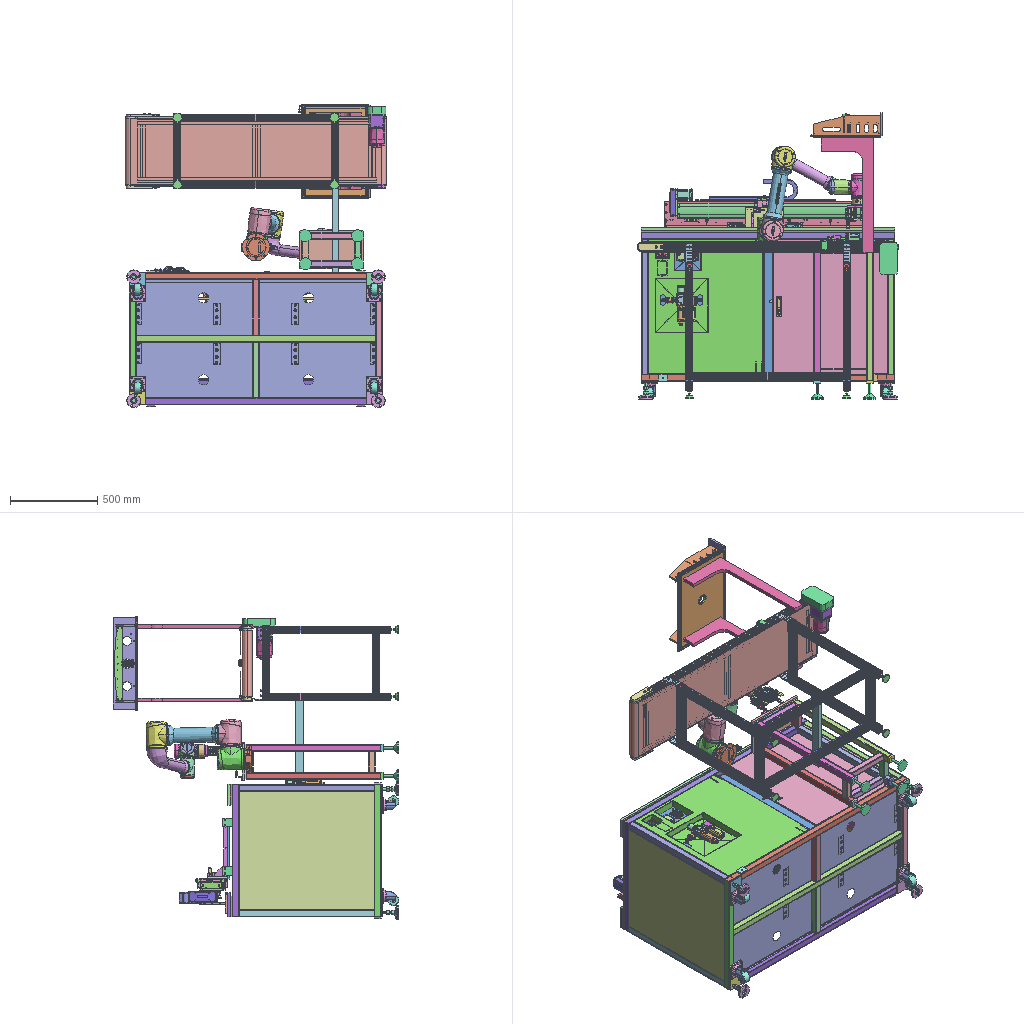Assembly | SolidWorks | 248 different items | 608 placed | box 1499 x 1641 x 1738 mm
Parts list (item | name | quantity | parent item | size | volume | features):
1 | (subassembly) | x2 | in 31 | 76 x 50 x 30 mm | 87070 mm3 | -
2 | (subassembly) | x1 | in 25 | 188 x 107.01 x 55 mm | 634944 mm3 | -
3 | (subassembly) | x1 | - | 112 x 47 x 54 mm | 166831 mm3 | -
4 | (subassembly) | x1 | in 24 | 35.5 x 35.5 x 68.5 mm | 34572 mm3 | -
5 | (subassembly) | x2 | in 14 | 435 x 890.5 x 50 mm | 1613187 mm3 | features ReferencePattern 5, CoordSys 2, AEMSimFeature 1, MirrorCompFeat 1, RefPoint 1
6 | (subassembly) | x2 | in 24 | 30 x 23 x 101 mm | 24926 mm3 | features AEMSimFeature 1
7 | (subassembly) | x1 | in 23 | 72 x 61 x 26 mm | 82860 mm3 | -
8 | (subassembly) | x1 | in 22 | - | - | features AEMSimFeature 1
9 | (subassembly) | x1 | - | 800 x 110 x 40.5 mm | 162817 mm3 | features LocalLPattern 1
10 | (subassembly) | x1 | in 25 | 1114 x 188.406 x 68 mm | 3201013 mm3 | -
11 | (subassembly) | x1 | in 34 | 20 x 9.65 x 39.9 mm | 1043 mm3 | -
12 | (subassembly) | x1 | in 10 | 1084 x 15 x 15 mm | 188228 mm3 | -
13 | (subassembly) | x8 | in 5 | 35.4 x 17.5 x 29.4 mm | 3403 mm3 | -
14 | (subassembly) | x1 | - | - | 14957387 mm3 | features CoordSys 3, ReferencePattern 3, LocalLPattern 2
15 | (subassembly) | x12 | in 17 | 13.848 x 23 x 26.25 mm | 3358 mm3 | -
16 | (subassembly) | x6 | in 14 | 13.848 x 23 x 26.25 mm | 3358 mm3 | -
17 | (subassembly) | x4 | in 5 | 70.833 x 123.25 x 40 mm | 44088 mm3 | features CompositeCurve 1
18 | (subassembly) | x6 | - | 41.5 x 411.771 x 715 mm | 1109076 mm3 | features ReferencePattern 2, LocalLPattern 1
19 | (subassembly) | x2 | in 24 | 50.042 x 30.664 x 10.3 mm | 4689 mm3 | -
20 | (subassembly) | x1 | in 31 | 669.522 x 661.013 x 466.347 mm | 12326745 mm3 | features CoordSys 7, RefAxis 6, RefPoint 6, AEMSimFeature 1, Attribute 1
21 | (subassembly) | x2 | in 32 | 190 x 40.32 x 40 mm | 18095 mm3 | -
22 | (subassembly) | x1 | - | - | - | features AEMSimFeature 1
23 | (subassembly) | x1 | in 32 | 49.5 x 90 x 200 mm | 386191 mm3 | -
24 | (subassembly) | x1 | - | - | 37015208 mm3 | features ReferencePattern 4, CompositeCurve 1, MirrorCompFeat 1
25 | (subassembly) | x1 | - | - | 11174306 mm3 | features ReferencePattern 5, LocalLPattern 1
26 | (subassembly) | x1 | - | - | 52361589 mm3 | features ReferencePattern 31, LocalLPattern 3, AEMSimFeature 1, CompositeCurve 1
27 | (subassembly) | x1 | - | - | 53088556 mm3 | features ReferencePattern 75, LocalLPattern 6, AEMSimFeature 1, CompositeCurve 1
28 | (subassembly) | x2 | - | - | 9390666 mm3 | features ReferencePattern 35, LocalLPattern 3, AEMSimFeature 1, CompositeCurve 1
29 | (subassembly) | x2 | in 31 | 117.707 x 64.465 x 76.746 mm | 74961 mm3 | -
30 | (subassembly) | x1 | - | 944.207 x 496.5 x 267 mm | 12174928 mm3 | features ReferencePattern 14, LocalLPattern 4, CompositeCurve 2
31 | (subassembly) | x1 | - | - | 12699341 mm3 | -
32 | (subassembly) | x1 | - | 370 x 949.5 x 230 mm | 4110556 mm3 | -
33 | (subassembly) | x4 | in 24 | 99.5 x 92 x 90 mm | 206753 mm3 | -
34 | (subassembly) | x1 | in 22 | 540 x 401 x 14.65 mm | 2063206 mm3 | -
35 | (subassembly) | x1 | in 22 | 63.129 x 47 x 47 mm | 44730 mm3 | -
36 | (subassembly) | x1 | in 24 | 72.5 x 225.5 x 124 mm | 471069 mm3 | features AEMSimFeature 1
37 | (subassembly) | x2 | in 29 | 85 x 53 x 27.5 mm | 63420 mm3 | -
38 | (subassembly) | x4 | in 25 | 86 x 50 x 30 mm | 87070 mm3 | -
39 | - | x1 | - | 44.5 x 12.5 x 450 mm | 69033 mm3 | features ICE 5, BossThin 2, LPattern 2, Chamfer 1, FlatPattern 1, SMBaseFlange 1, SheetMetal 1
40 | - | x12 | in 18 | 120 x 40 x 8 mm | 35212 mm3 | features 3DProfileFeature 2, HoleWzd 2, Chamfer 1, Extrusion 1
41 | - | x1 | in 35 | 3.978 x 6.858 x 6.442 mm | 52.243 mm3 | features BaseBody 1
42 | - | x1 | in 35 | 11.433 x 39.8 x 39.8 mm | 7338 mm3 | features BaseBody 1
43 | - | x1 | in 35 | 3.5 x 2.5 x 2.5 mm | 6.379 mm3 | features BaseBody 1
44 | - | x1 | in 35 | 3.5 x 2.5 x 2.5 mm | 6.379 mm3 | features BaseBody 1
45 | - | x1 | in 35 | - | - | features RefSurface 1
46 | - | x1 | in 35 | - | - | features RefSurface 1
47 | - | x1 | in 35 | - | - | features RefSurface 1
48 | - | x1 | in 35 | 38.251 x 31 x 31 mm | 8383 mm3 | features BaseBody 1
49 | - | x1 | in 35 | - | - | features RefSurface 1
50 | - | x3 | in 10 | 25 x 19 x 16 mm | 1321 mm3 | features BaseBody 1
51 | - | x1 | in 35 | - | - | features RefSurface 1
52 | - | x1 | in 35 | - | - | features RefSurface 1
53 | - | x1 | in 35 | 3.978 x 6.905 x 6.388 mm | 52.243 mm3 | features BaseBody 1
54 | - | x1 | in 35 | 9.2 x 37.648 x 37.599 mm | 107.29 mm3 | features BaseBody 1
55 | - | x1 | in 35 | - | - | features RefSurface 1
56 | - | x1 | in 35 | - | - | features RefSurface 1
57 | - | x1 | in 35 | 14.76 x 38.6 x 38.577 mm | 3869 mm3 | features BaseBody 1
58 | - | x1 | in 35 | - | - | features RefSurface 1
59 | - | x1 | in 35 | 7 x 22 x 22 mm | 502.064 mm3 | features BaseBody 1
60 | - | x1 | in 35 | - | - | features RefSurface 1
61 | - | x1 | - | 80 x 78.941 x 69 mm | 302744 mm3 | features Chamfer 2, Extrusion 1, ICE 1
62 | - | x1 | in 35 | 1.6 x 1.946 x 2.281 mm | 2.431 mm3 | features BaseBody 1
63 | - | x1 | in 35 | 3.031 x 17.3 x 17.3 mm | 416.795 mm3 | features BaseBody 1
64 | - | x1 | in 35 | 3.5 x 2.5 x 2.5 mm | 6.379 mm3 | features BaseBody 1
65 | - | x1 | in 35 | 12.2 x 38.6 x 38.6 mm | 2092 mm3 | features BaseBody 1
66 | - | x1 | in 35 | 1.6 x 2.017 x 2.199 mm | 2.431 mm3 | features BaseBody 1
67 | - | x1 | in 35 | 2.5 x 3.555 x 6.804 mm | 24.947 mm3 | features BaseBody 1
68 | - | x1 | in 35 | 1.6 x 2.26 x 1.67 mm | 2.431 mm3 | features BaseBody 1
69 | - | x1 | - | 20 x 67.5 x 20 mm | 8070 mm3 | features Revolution 1
70 | - | x2 | in 24 | 35.315 x 37 x 18 mm | 6709 mm3 | features BaseBody 1
71 | - | x1 | - | - | - | features RefSurface 21
72 | - | x4 | in 14 | 62.36 x 40 x 17.8 mm | 10187 mm3 | features BaseBody 1
73 | - | x1 | in 24 | 1453 x 880 x 780 mm | 27439038 mm3 | features HoleWzd 6, ICE 5, FlatPattern 3, SMBaseFlange 3, SheetMetal 3, EdgeFlange 2, 3DProfileFeature 1, MirrorPattern 1, MoveFace 1, WeldMemberFeat 1, WeldmentFeature 1
74 | - | x1 | in 24 | 667.5 x 46.5 x 774 mm | 968316 mm3 | features EdgeFlange 8, ICE 6, FlatPattern 5, HoleWzd 3, SMBaseFlange 2, SMWeldBead 2, SheetMetal 2, MirrorPattern 1, MirrorSolid 1
75 | - | x1 | in 24 | 659 x 10.5 x 779 mm | 836638 mm3 | features SMWeldBead 4, EdgeFlange 2, FlatPattern 1, HoleWzd 1, ICE 1, SMBaseFlange 1, SheetMetal 1
76 | - | x1 | in 24 | 65 x 65 x 104.965 mm | 219842 mm3 | features BaseBody 9
77 | - | x3 | in 26, 28 | 75 x 62 x 80 mm | 102466 mm3 | features Fillet 2, HoleWzd 2, Extrusion 1, Revolution 1
78 | - | x1 | in 10 | 159 x 62 x 34.528 mm | 50117 mm3 | features BaseBody 1
79 | - | x1 | in 10 | 159 x 62 x 12 mm | 73972 mm3 | features BaseBody 1
80 | - | x1 | in 10 | 85 x 64 x 23 mm | 64137 mm3 | features BaseBody 1
81 | - | x1 | in 10 | 84 x 8.038 x 1060 mm | 538813 mm3 | features BaseBody 1
82 | - | x1 | in 12 | 1084 x 15 x 15 mm | 188228 mm3 | features BaseBody 1
83 | - | x56 | in 28 | 62.36 x 40 x 17.8 mm | 10187 mm3 | features BaseBody 1
84 | - | x1 | in 10 | 85 x 64 x 18 mm | 62222 mm3 | features BaseBody 1
85 | - | x1 | in 10 | 86 x 38.5 x 1040 mm | 1661800 mm3 | features BaseBody 1
86 | - | x1 | in 10 | 114.08 x 56 x 105 mm | 257643 mm3 | features BaseBody 1
87 | - | x1 | in 25 | - | - | features RefSurface 2
88 | - | x1 | - | - | - | features RefSurface 8
89 | - | x2 | in 5 | 425 x 730.5 x 40 mm | 1437708 mm3 | features ICE 3, WeldMemberFeat 1, WeldmentFeature 1
90 | - | x1 | in 14 | 51.5 x 1389 x 400 mm | 4308488 mm3 | features ICE 1, WeldMemberFeat 1, WeldmentFeature 1
91 | - | x1 | in 14 | 425 x 861 x 40 mm | 1154541 mm3 | features CoordSys 1, WeldMemberFeat 1, WeldmentFeature 1
92 | - | x8 | in 13 | 14 x 14 x 29.4 mm | 1691 mm3 | features ICE 2, RevCut 2, Chamfer 1, Extrusion 1
93 | - | x4 | in 5 | 40 x 40 x 9 mm | 3574 mm3 | features BaseBody 1
94 | - | x8 | in 13 | 35.4 x 16.108 x 17.5 mm | 1712 mm3 | features BaseBody 1
95 | - | x12 | in 15 | 13.848 x 23 x 8.25 mm | 1654 mm3 | features Extrusion 1, HoleWzd 1, Revolution 1
96 | - | x6 | in 16 | 13.848 x 23 x 8.25 mm | 1654 mm3 | features Extrusion 1, HoleWzd 1, Revolution 1
97 | - | x1 | in 14 | 426 x 55 x 152.5 mm | 1121917 mm3 | features ICE 2, Chamfer 1, Extrusion 1, HoleWzd 1, MirrorPattern 1
98 | - | x1 | in 14 | 468 x 187.5 x 152.5 mm | 2041329 mm3 | features ICE 8, Chamfer 1, Extrusion 1, HoleWzd 1
99 | - | x12 | in 15 | 13 x 13 x 24 mm | 1703 mm3 | features ICE 2, Chamfer 1, Extrusion 1, Fillet 1, RevCut 1
100 | - | x6 | in 16 | 13 x 13 x 24 mm | 1703 mm3 | features ICE 2, Chamfer 1, Extrusion 1, Fillet 1, RevCut 1
101 | - | x4 | in 5 | 50 x 82.6 x 50 mm | 33276 mm3 | features BaseBody 1
102 | - | x3 | in 14 | 21.5 x 16 x 40 mm | 4531 mm3 | features BaseBody 3, ICE 1
103 | - | x4 | in 17 | 70 x 110 x 40 mm | 34015 mm3 | features ICE 3, Fillet 2, MoveFace 2, BaseBody 1
104 | - | x4 | in 33 | 42 x 13 x 13 mm | 5217 mm3 | features RefAxis 6, 3DProfileFeature 2, Revolution 1
105 | - | x28 | in 26, 28 | 380 x 380 x 20 mm | 1730652 mm3 | features Fillet 3, ICE 2, Extrusion 1, LPattern 1
106 | - | x2 | in 19 | 39.8 x 19.1 x 10.3 mm | 4486 mm3 | features ICE 8, Chamfer 4, Extrusion 1, MirrorPattern 1
107 | - | x2 | in 19 | 29.3 x 10.5 x 6.4 mm | 172.618 mm3 | features ICE 5, Fillet 3, Chamfer 2, Extrusion 1
108 | - | x2 | in 19 | 1.5 x 5 x 4.3 mm | 30.174 mm3 | features Extrusion 1
109 | - | x1 | in 24 | 71.998 x 25.1 x 117 mm | 44510 mm3 | features BaseBody 1
110 | - | x1 | in 20 | - | - | features RefAxis 3, BaseBody 2, RefSurface 2, CoordSys 1
111 | - | x1 | in 20 | 126.523 x 157.65 x 125.047 mm | 1928290 mm3 | features BaseBody 1
112 | - | x1 | in 20 | 555.047 x 157.65 x 125.047 mm | 5841153 mm3 | features BaseBody 3
113 | - | x1 | in 20 | 469.687 x 125 x 118 mm | 2299824 mm3 | features BaseBody 3, Fillet 1, ICE 1, RefAxis 1, RefPoint 1
114 | - | x1 | in 20 | 87.688 x 125 x 84.375 mm | 705522 mm3 | features BaseBody 2, Fillet 1, ICE 1
115 | - | x4 | in 33 | 66 x 58.3 x 58 mm | 18491 mm3 | features RefAxis 15, ICE 6, 3DProfileFeature 5, Revolution 2
116 | - | x1 | in 20 | 87.688 x 143.092 x 84.375 mm | 806898 mm3 | features BaseBody 2
117 | - | x1 | in 20 | 81 x 39 x 81.209 mm | 180493 mm3 | features BaseBody 2
118 | - | x1 | in 4 | 35.5 x 35.5 x 39 mm | 15226 mm3 | features BaseBody 1
119 | - | x1 | in 4 | 25.403 x 22.74 x 68.5 mm | 19346 mm3 | features BaseBody 1
120 | - | x2 | in 7 | 7 x 8.083 x 6.5 mm | 169.1 mm3 | features BaseBody 1
121 | - | x1 | in 7 | 26 x 58 x 59 mm | 66281 mm3 | features BaseBody 1
122 | - | x1 | in 7 | 22 x 56 x 67.5 mm | 16241 mm3 | features BaseBody 1
123 | - | x1 | in 32 | 365 x 15 x 220 mm | 1203750 mm3 | features BaseBody 1
124 | - | x1 | in 32 | 340 x 795 x 200 mm | 2102526 mm3 | features BaseBody 20, MoveFace 1
125 | - | x1 | in 34 | 62 x 62 x 9 mm | 6673 mm3 | features BaseBody 1
126 | - | x4 | in 33 | 58.511 x 2 x 58.511 mm | 5378 mm3 | features RefAxis 9, 3DProfileFeature 3, Revolution 1
127 | - | x1 | in 34 | 518 x 360 x 5 mm | 918757 mm3 | features BaseBody 1
128 | - | x1 | in 34 | 540 x 382 x 3 mm | 612788 mm3 | features BaseBody 1
129 | - | x2 | in 14 | 160.77 x 37.32 x 13.1 mm | 7719 mm3 | features BaseBody 2
130 | - | x2 | in 21 | 160.77 x 37.32 x 13.1 mm | 7719 mm3 | features BaseBody 2
131 | - | x2 | in 21 | 38 x 40 x 57 mm | 10376 mm3 | features BaseBody 1
132 | - | x1 | in 23 | 15 x 50 x 105 mm | 61072 mm3 | features BaseBody 1
133 | - | x1 | in 23 | 10 x 90 x 200 mm | 179500 mm3 | features BaseBody 1
134 | - | x1 | in 23 | 8.4 x 35 x 36.4 mm | 6248 mm3 | features BaseBody 1
135 | - | x1 | in 23 | 8.8 x 22 x 56 mm | 10314 mm3 | features BaseBody 1
136 | - | x1 | in 34 | 514.4 x 356.4 x 2 mm | 361307 mm3 | features BaseBody 1
137 | - | x4 | in 33 | 90 x 14.2 x 90 mm | 60346 mm3 | features RefAxis 6, 3DProfileFeature 2, ICE 2, Extrusion 1, Revolution 1
138 | - | x1 | in 23 | 13.5 x 59 x 58 mm | 46197 mm3 | features BaseBody 1
139 | - | x1 | in 34 | 20 x 374 x 9 mm | 32363 mm3 | features BaseBody 1
140 | - | x1 | in 34 | 20 x 374 x 9 mm | 32363 mm3 | features BaseBody 1
141 | - | x1 | in 34 | 540 x 20 x 9 mm | 48939 mm3 | features BaseBody 1
142 | - | x1 | in 34 | 540 x 20 x 9 mm | 48974 mm3 | features BaseBody 1
143 | - | x1 | in 24 | 1453 x 120 x 15 mm | 2605469 mm3 | features 3DProfileFeature 2, HoleWzd 2, Chamfer 1, Extrusion 1
144 | - | x1 | in 24 | 1400 x 140 x 15 mm | 2905465 mm3 | features HoleWzd 3, 3DProfileFeature 2, Chamfer 1, Extrusion 1, LPattern 1
145 | - | x3 | in 26, 28 | 154 x 46 x 10 mm | 7085 mm3 | features ExtruThin 1
146 | - | x1 | - | 47 x 28 x 13 mm | 6727 mm3 | features HoleWzd 2, ICE 2, Extrusion 1
147 | - | x1 | - | 60 x 812.195 x 122 mm | 146456 mm3 | features EdgeFlange 5, FlatPattern 2, ICE 2, SMBaseFlange 2, SheetMetal 2
148 | - | x1 | - | 36 x 124 x 438 mm | 261522 mm3 | features ICE 1, Sweep 1
149 | - | x4 | in 33 | 38 x 65 x 65 mm | 117321 mm3 | features RefAxis 9, 3DProfileFeature 3, Revolution 1
150 | - | x3 | in 26, 28 | 106 x 80 x 63 mm | 286934 mm3 | features BaseBody 39
151 | - | x4 | in 25 | 50 x 85 x 17 mm | 54838 mm3 | features Extrusion 1, HoleWzd 1, ICE 1
152 | - | x1 | - | 500 x 845 x 500 mm | 14590958 mm3 | features BaseBody 6, MoveFace 1
153 | - | x4 | in 29 | 49 x 20 x 10 mm | 5771 mm3 | features ICE 4, Chamfer 2, Extrusion 1, HoleWzd 1, MoveFace 1
154 | - | x1 | - | 103 x 10 x 54 mm | 11241 mm3 | features HoleWzd 1, Sweep 1
155 | - | x1 | in 25 | 63 x 124 x 504 mm | 448072 mm3 | features ICE 1, Sweep 1
156 | - | x3 | in 26, 28 | 106 x 80 x 30 mm | 171843 mm3 | features BaseBody 19
157 | - | x1 | - | - | - | features RefSurface 1
158 | - | x3 | in 26, 28 | - | - | features RefSurface 3
159 | - | x1 | - | - | - | features RefSurface 4
160 | - | x2 | in 14 | 30 x 30 x 48 mm | 4472 mm3 | features EdgeFlange 1, Fillet 1, FlatPattern 1, SMBaseFlange 1, SheetMetal 1
161 | - | x1 | - | 30 x 483.5 x 50 mm | 725250 mm3 | features Extrusion 1
162 | - | x1 | - | 172.7 x 60 x 15 mm | 14511 mm3 | features BaseBody 1
163 | - | x3 | in 26, 28 | 24.985 x 38.085 x 10.8 mm | 6244 mm3 | features ICE 7, Revolution 7, Extrusion 1, HoleWzd 1
164 | - | x3 | in 26, 28 | - | - | features RefSurface 10
165 | - | x3 | in 10 | 13 x 15.5 x 39.5 mm | 3396 mm3 | features BaseBody 2
166 | - | x9 | in 26, 28 | 13.6 x 15.5 x 27.7 mm | 2033 mm3 | features BaseBody 1
167 | - | x1 | in 36 | 50.45 x 124.7 x 47.5 mm | 63459 mm3 | features ICE 7, RefAxis 3, Revolution 2, 3DProfileFeature 1
168 | - | x1 | in 36 | 56.1 x 88 x 12.5 mm | 22912 mm3 | features RefAxis 12, 3DProfileFeature 4, ICE 3, Extrusion 1
169 | - | x1 | in 36 | 4.4 x 49.3 x 12.5 mm | 2160 mm3 | features RefAxis 9, 3DProfileFeature 3, RevCut 2, Extrusion 1, ICE 1
170 | - | x2 | in 36 | 11 x 8.5 x 8.5 mm | 289.091 mm3 | features RefAxis 3, 3DProfileFeature 1, ICE 1, Revolution 1
171 | - | x2 | in 22 | 20 x 300 x 660 mm | 1191451 mm3 | features Extrusion 1, Fillet 1, ICE 1
172 | - | x1 | in 36 | 57.7 x 52 x 60 mm | 115730 mm3 | features RefAxis 18, ICE 7, 3DProfileFeature 6, RevCut 3, Extrusion 1
173 | - | x1 | in 36 | 50.45 x 106.5 x 47.5 mm | 58230 mm3 | features ICE 7, RefAxis 3, 3DProfileFeature 1, Revolution 1
174 | - | x1 | in 36 | 53.5 x 148.9 x 60 mm | 120661 mm3 | features RefAxis 9, ICE 8, 3DProfileFeature 3, RevCut 3, Extrusion 1, Revolution 1
175 | - | x1 | in 36 | 53.4 x 61.5 x 51 mm | 87339 mm3 | features ICE 5, RefAxis 3, Revolution 2, 3DProfileFeature 1, Extrusion 1
176 | - | x1 | in 24 | 52 x 33.3 x 71.95 mm | 53395 mm3 | features BaseBody 12
177 | - | x1 | in 24 | 52 x 45 x 71.95 mm | 42694 mm3 | features BaseBody 10
178 | - | x1 | - | - | - | features RefSurface 48
179 | - | x2 | in 37 | 62.5 x 53 x 27.5 mm | 57393 mm3 | features BaseBody 1
180 | - | x2 | in 37 | 27.3 x 19.4 x 15.5 mm | 3013 mm3 | features BaseBody 1
181 | - | x2 | in 37 | 27.3 x 19.4 x 15.5 mm | 3013 mm3 | features BaseBody 1
182 | - | x1 | in 31 | 65 x 130 x 8 mm | 50920 mm3 | features Chamfer 1, Extrusion 1, ICE 1
183 | - | x3 | in 26, 28 | 48 x 34.5 x 84 mm | 100896 mm3 | features ICE 12, HoleWzd 5, RevCut 4, Chamfer 3, Draft 3, Extrusion 1, Fillet 1
184 | - | x6 | in 26, 28 | 23 x 22 x 780 mm | 325761 mm3 | features ICE 6, Draft 4, Chamfer 2, HoleWzd 2, Extrusion 1, LPattern 1
185 | - | x6 | in 1, 38 | 75 x 49.9 x 28.55 mm | 42408 mm3 | features BaseBody 1
186 | - | x6 | in 1, 38 | 66 x 50 x 21.5 mm | 44662 mm3 | features BaseBody 1
187 | - | x1 | in 2 | 156 x 106.01 x 50.5 mm | 274735 mm3 | features BaseBody 1
188 | - | x1 | in 2 | 179.95 x 107 x 54.1 mm | 360209 mm3 | features BaseBody 1
189 | - | x1 | - | 112 x 47 x 54 mm | 166831 mm3 | features BaseBody 1
190 | - | x3 | in 26, 28 | 16 x 48 x 48 mm | 14625 mm3 | features ICE 3, Fillet 2, HoleWzd 2, BaseBody 1, RevCut 1
191 | - | x2 | in 22 | 382 x 10 x 115 mm | 327144 mm3 | features HoleWzd 4, ICE 3, LPattern 2, Chamfer 1, Cut 1, Extrusion 1, MoveFace 1
192 | - | x1 | in 22 | 530 x 130 x 10 mm | 625792 mm3 | features HoleWzd 2, Chamfer 1, Cut 1, Extrusion 1, Fillet 1, LPattern 1
193 | - | x2 | in 31 | 50 x 70 x 8 mm | 28000 mm3 | features Extrusion 1
194 | - | x1 | in 22 | 426 x 10 x 50 mm | 182893 mm3 | features HoleWzd 3, Chamfer 2, MirrorPattern 2, Extrusion 1
195 | - | x1 | - | 42 x 42 x 30 mm | 12218 mm3 | features Extrusion 1, HoleWzd 1, ICE 1
196 | - | x2 | in 6 | 30 x 23 x 67 mm | 16541 mm3 | features ICE 4, Extrusion 1, Fillet 1, HoleWzd 1
197 | - | x2 | in 6 | 86.5 x 14 x 16 mm | 5306 mm3 | features Chamfer 1, ICE 1, Revolution 1
198 | - | x2 | in 6 | 30 x 15 x 14 mm | 3079 mm3 | features Extrusion 1, HoleWzd 1, ICE 1
199 | - | x4 | in 24 | 80 x 178.5 x 80 mm | 123669 mm3 | features HoleWzd 2, Revolution 2, Fillet 1, ICE 1, LPattern 1, RevCut 1
200 | - | x4 | in 32 | 70 x 150 x 70 mm | 95473 mm3 | features BaseBody 1
201 | - | x1 | in 10 | 118 x 65.906 x 60 mm | 289861 mm3 | features BaseBody 1
202 | - | x1 | in 8 | - | - | features BaseBody 11, RefSurface 1
203 | - | x1 | - | 450 x 15 x 40 mm | 179202 mm3 | features HoleWzd 2, Extrusion 1
204 | - | x1 | in 11 | 10 x 9.65 x 30.024 mm | 791.952 mm3 | features BaseBody 1
205 | - | x1 | - | 460 x 40 x 40 mm | 111480 mm3 | features HoleWzd 2, EdgeFlange 1, FlatPattern 1, SMBaseFlange 1, SheetMetal 1
206 | - | x1 | - | 460 x 40 x 4 mm | 73267 mm3 | features Extrusion 1, HoleWzd 1
207 | - | x1 | - | 40 x 53.5 x 59 mm | 6153 mm3 | features EdgeFlange 2, FlatPattern 1, ICE 1, SMBaseFlange 1, SheetMetal 1
208 | - | x1 | - | 12 x 242 x 460 mm | 1328431 mm3 | features HoleWzd 5, Extrusion 1, MirrorPattern 1
209 | - | x1 | - | 68 x 100 x 10 mm | 24328 mm3 | features HoleWzd 3, Extrusion 1
210 | - | x1 | - | 80 x 10 x 460 mm | 360747 mm3 | features HoleWzd 2, Extrusion 1
211 | - | x1 | - | 320 x 320 x 10 mm | 1021792 mm3 | features HoleWzd 2, MirrorPattern 2, Extrusion 1
212 | - | x1 | - | 12 x 12 x 200 mm | 22610 mm3 | features Chamfer 1, Extrusion 1
213 | - | x1 | - | 320 x 320 x 12 mm | 1198946 mm3 | features HoleWzd 4, MirrorPattern 2, Extrusion 1
214 | - | x1 | - | 430 x 12 x 12 mm | 58809 mm3 | features HoleWzd 2, Extrusion 1, ICE 1
215 | - | x1 | in 11 | 16.9 x 3.8 x 10.488 mm | 251.226 mm3 | features BaseBody 1
216 | - | x1 | - | 38 x 16 x 2 mm | 1034 mm3 | features FlatPattern 1, HoleWzd 1, SMBaseFlange 1, SheetMetal 1
217 | - | x1 | - | 50 x 20 x 50 mm | 8727 mm3 | features EdgeFlange 1, FlatPattern 1, HoleWzd 1, ICE 1, SMBaseFlange 1, SheetMetal 1
218 | - | x1 | - | 550 x 45 x 10 mm | 65036 mm3 | features EdgeFlange 1, FlatPattern 1, HoleWzd 1, ICE 1, SMBaseFlange 1, SheetMetal 1
219 | - | x1 | - | 78 x 30 x 22.5 mm | 5453 mm3 | features EdgeFlange 2, FlatPattern 1, HoleWzd 1, ICE 1, SMBaseFlange 1, SheetMetal 1
220 | - | x1 | - | 190 x 50 x 14.5 mm | 135905 mm3 | features Extrusion 1
221 | - | x6 | in 26, 28 | 390 x 60 x 12 mm | 149830 mm3 | features HoleWzd 3, 3DProfileFeature 1, Extrusion 1, LPattern 1
222 | - | x6 | in 26, 28 | 400 x 30 x 15 mm | 159842 mm3 | features 3DProfileFeature 2, HoleWzd 2, Extrusion 1
223 | - | x3 | in 26, 28 | 410 x 110 x 12 mm | 516360 mm3 | features 3DProfileFeature 3, HoleWzd 3, ICE 2, LPattern 2, Extrusion 1
224 | - | x3 | in 26, 28 | 90 x 75 x 60 mm | 256657 mm3 | features 3DProfileFeature 2, HoleWzd 2, Chamfer 1, Extrusion 1
225 | - | x3 | in 26, 28 | 40 x 43.5 x 15 mm | 3159 mm3 | features EdgeFlange 2, FlatPattern 1, ICE 1, SMBaseFlange 1, SheetMetal 1
226 | - | x12 | in 18 | 40 x 80 x 4 mm | 11536 mm3 | features 3DProfileFeature 1, Chamfer 1, Extrusion 1, HoleWzd 1
227 | - | x3 | in 26, 28 | 85 x 85 x 38 mm | 42909 mm3 | features ICE 2, 3DProfileFeature 1, Extrusion 1, HoleWzd 1
228 | - | x6 | in 26, 28 | 36 x 53.5 x 794 mm | 1434418 mm3 | features HoleWzd 4, Extrusion 1, LPattern 1
229 | - | x9 | in 26, 28 | 29 x 22 x 22 mm | 1498 mm3 | features 3DProfileFeature 1, EdgeFlange 1, FlatPattern 1, HoleWzd 1, SMBaseFlange 1, SheetMetal 1
230 | - | x3 | in 26, 28 | 30 x 30.001 x 630 mm | 208708 mm3 | features 3DProfileFeature 1, Extrusion 1, HoleWzd 1
231 | - | x3 | in 26, 28 | 20 x 25 x 35 mm | 1305 mm3 | features EdgeFlange 1, Fillet 1, FlatPattern 1, ICE 1, SMBaseFlange 1, SheetMetal 1
232 | - | x3 | in 26, 28 | 32 x 734 x 32 mm | 548270 mm3 | features ICE 4, Chamfer 1, RevCut 1, Revolution 1
233 | - | x1 | - | 140 x 15 x 20 mm | 15054 mm3 | features ICE 3, Chamfer 2, Extrusion 1
234 | - | x1 | in 25 | 350 x 366 x 10 mm | 802882 mm3 | features ICE 3, 3DProfileFeature 1, Extrusion 1, HoleWzd 1, LPattern 1
235 | - | x2 | in 25 | 320 x 90 x 12 mm | 122776 mm3 | features 3DProfileFeature 2, HoleWzd 2, Extrusion 1
236 | - | x1 | in 25 | 220 x 12 x 120 mm | 304867 mm3 | features HoleWzd 6, 3DProfileFeature 3, Extrusion 1
237 | - | x1 | in 14 | - | - | features BaseBody 6, CoordSys 1, ICE 1, RefSurface 1
238 | - | x1 | in 25 | 120 x 140 x 12 mm | 195775 mm3 | features HoleWzd 3, 3DProfileFeature 2, Extrusion 1, ICE 1, MirrorPattern 1
239 | - | x1 | in 25 | 1200 x 140 x 15 mm | 2477276 mm3 | features HoleWzd 4, LPattern 4, 3DProfileFeature 1, Extrusion 1
240 | - | x1 | - | 140 x 130 x 15 mm | 95031 mm3 | features 3DProfileFeature 1, Extrusion 1, HoleWzd 1
241 | - | x1 | in 25 | 1200 x 120 x 15 mm | 2114705 mm3 | features 3DProfileFeature 2, HoleWzd 2, Extrusion 1, ICE 1
242 | - | x1 | - | 30 x 218 x 20.5 mm | 20090 mm3 | features EdgeFlange 3, FlatPattern 1, HoleWzd 1, ICE 1, SMBaseFlange 1, SheetMetal 1
243 | - | x1 | in 25 | 800 x 80 x 10 mm | 150971 mm3 | features EdgeFlange 1, FlatPattern 1, ICE 1, SMBaseFlange 1, SheetMetal 1
244 | - | x1 | - | 110 x 30 x 30.5 mm | 11846 mm3 | features EdgeFlange 2, FlatPattern 1, ICE 1, SMBaseFlange 1, SheetMetal 1
245 | - | x6 | in 18 | 411.771 x 517 x 8.423 mm | 269565 mm3 | features EdgeFlange 1, FlatPattern 1, ICE 1, SMBaseFlange 1, SheetMetal 1
246 | - | x6 | in 18 | 40 x 80 x 300 mm | 325543 mm3 | features 3DProfileFeature 2, HoleWzd 2, Extrusion 1
247 | - | x12 | in 18 | 40 x 80 x 190 mm | 210236 mm3 | features 3DProfileFeature 1, Extrusion 1, HoleWzd 1
248 | - | x1 | - | 24 x 71 x 375.5 mm | 114976 mm3 | features ICE 2, Sweep 1
Mates (type | each side: item.copy, entity, surface, feature), first 389 of 498 lines:
In the top assembly
Coincident | 144.1 face plane Boss-Extrude 1 | 241.1 face plane Boss-Extrude 1 | 2 times
DistanceDim | 241.1 face plane Boss-Extrude 1 | 144.1 face plane Boss-Extrude 1
Coincident | 73.1 face plane Boss-Extrude 6 | 228.1 face plane Boss-Extrude 1
DistanceDim | 228.1 face plane Boss-Extrude 1 | 143.1 face plane Boss-Extrude 1
Coincident | 73.1 face plane Boss-Extrude 6 | 228.2 face plane Boss-Extrude 1
Coincident | 228.3 face plane Boss-Extrude 1 | 228.2 face plane Boss-Extrude 1
Coincident | 73.1 face plane Base-Flange 1 | 40.1 face plane Boss-Extrude 1
Coincident | 73.1 face plane Base-Flange 1 | 40.2 face plane Boss-Extrude 1
Coincident | 226.1 face plane Boss-Extrude 1 | 226.2 face plane Boss-Extrude 1
Width | 245.1 face plane Base-Flange 1 | 245.2 face plane Base-Flange 1 | 221.1 face plane Boss-Extrude 1 | 221.2 face plane Boss-Extrude 1
DistanceDim | 245.1 face plane Base-Flange 1 | 245.2 face plane Base-Flange 1
Coincident | 73.1 face plane Base-Flange 1 | 40.3 face plane Boss-Extrude 1
Coincident | 246.1 face plane Boss-Extrude 1 | 246.2 face plane Boss-Extrude 1
Coincident | 226.3 face plane Boss-Extrude 1 | 226.4 face plane Boss-Extrude 1
DistanceDim | 245.3 face plane Base-Flange 1 | 245.4 face plane Base-Flange 1
Coincident | 226.1 face plane Boss-Extrude 1 | 226.3 face plane Boss-Extrude 1
Width | 245.4 face plane Base-Flange 1 | 245.3 face plane Base-Flange 1 | 221.3 face plane Boss-Extrude 1 | 221.4 face plane Boss-Extrude 1
Coincident | 199.1 face plane Revolve 1 | assembly face
Coincident | 199.1 face plane Revolve 1 | 200.1 face plane  Import 1
Coincident | 199.1 face plane Revolve 1 | 101.1 face plane  Import 1
Width | 171.1 face plane Boss-Extrude 1 | 171.2 face plane Boss-Extrude 1 | 90.1 face plane LE-8-5050W | 90.1 face plane LE-8-5050W
Width | 73.1 face plane  C:\xxxxxxxxxxxxxxxxxx\xx\xxxx\xxxxxxxxxxxxxxxx | 73.1 face plane  C:\xxxxxxxxxxxxxxxxxx\xx\xxxx\xxxxxxxxxxxxxxxx | 89.1 face plane LE-8-4040HW | 89.2 face plane LE-8-4040HW
DistanceDim | 89.2 face plane LE-8-4040HW | 171.1 face plane Cut-Extrude 1
Coincident | 73.1 face plane  C:\xxxxxxxxxxxxxxxxxx\xx\xxxx\xxxxxxxxxxxxxxxx | assembly face
Width | 73.1 face plane  C:\xxxxxxxxxxxxxxxxxx\xx\xxxx\xxxxxxxxxxxxxxxx | 73.1 face plane  C:\xxxxxxxxxxxxxxxxxx\xx\xxxx\xxxxxxxxxxxxxxxx | assembly face | assembly face
DistanceDim | 124.1 face plane  Import 6 | 73.1 face plane  C:\xxxxxxxxxxxxxxxxxx\xx\xxxx\xxxxxxxxxxxxxxxx
DistanceDim | 90.1 face plane LE-8-5050W | 73.1 face plane  C:\xxxxxxxxxxxxxxxxxx\xx\xxxx\xxxxxxxxxxxxxxxx
DistanceDim | 124.1 face plane  Import 8 | 73.1 face plane  C:\xxxxxxxxxxxxxxxxxx\xx\xxxx\xxxxxxxxxxxxxxxx
Coincident | 184.1 face plane Boss-Extrude 2 | 184.2 face plane Boss-Extrude 3
Coincident | 184.1 face plane Boss-Extrude 1 | 184.2 face plane Boss-Extrude 1
DistanceDim | 228.4 face plane Boss-Extrude 1 | 228.5 face plane Boss-Extrude 1
Coincident | 247.1 face plane Boss-Extrude 1 | 246.2 face plane Boss-Extrude 1
DistanceDim | 228.1 face plane Boss-Extrude 1 | 73.1 face plane  C:\xxxxxxxxxxxxxxxxxx\xx\xxxx\xxxxxxxxxxxxxxxx
DistanceDim | 247.2 face plane Boss-Extrude 1 | 73.1 face plane Boss-Extrude 6
Parallel | 143.1 face plane Boss-Extrude 1 | 182.1 face plane Boss-Extrude 2
Coincident | 89.2 face plane LE-8-4040HW | 161.1 face plane Boss-Extrude 1 | 2 times
In subassembly 18
Concentric | 247.3 face cylinder Boss-Extrude 1 | 40.4 face cylinder  Drill Hole Size (% per Cross ) Slotted Countersunk Wood Screw Type 1 | 2 times
Coincident | 247.3 face plane Boss-Extrude 1 | 40.4 face plane Boss-Extrude 1
Coincident | 247.3 face plane Boss-Extrude 1 | 246.3 face plane Boss-Extrude 1 | 2 times
Coincident | 245.5 face plane Base-Flange 1 | 246.3 face plane Boss-Extrude 1 | 2 times
DistanceDim | 246.3 face plane Boss-Extrude 1 | 245.5 edge
Concentric | 247.3 face cylinder Boss-Extrude 1 | 246.3 face cylinder  Drill Hole Size (% per ) Hex Socket Head Cap Screw Type 2
Coincident | 246.3 face plane Boss-Extrude 1 | 226.5 face plane Boss-Extrude 1 | 3 times
Coincident | 246.3 face plane Boss-Extrude 1 | 226.6 face plane Boss-Extrude 1 | 3 times
In subassembly 24
DistanceDim | 73.2 face plane  C:\xxxxxxxxxxxxxxxxxx\xx\xxxx\xxxxxxxxxxxxxxxx | 74.1 face plane Edge-Flange 1
Concentric | 73.2 face cylinder Ø6.2 (6.2) DiameterHole 1 | 74.1 face cylinder Ø6.0 (6) DiameterHole 1
LimitPlanarAngleDim | 74.1 face plane Base-Flange 1 | 73.2 face plane  C:\xxxxxxxxxxxxxxxxxx\xx\xxxx\xxxxxxxxxxxxxxxx
Concentric | 74.1 face cylinder Cut-Extrude 3 | 76.1 face cylinder  Import 8 | 2 times
Coincident | 74.1 face plane Edge-Flange 4 | 76.1 face plane  Import 3
Concentric | 74.1 face cylinder M3 Tapped Hole 1 | 196.1 face cylinder  Drill Hole Size Slotted Raised Countersunk Screw Type 1 | 2 times
Coincident | 74.1 face plane Base-Flange 2 | 196.1 face plane Boss-Extrude 1
Coincident | 74.1 face plane Mirror 1 | 196.2 face plane Boss-Extrude 1
Concentric | 74.1 face cylinder Mirror 5 | 196.2 face cylinder  Drill Hole Size Slotted Raised Countersunk Screw Type 1 | 2 times
Concentric | 73.2 face cylinder M3 Tapped Hole 1 | 106.1 face cylinder Cut-Extrude 1
Coincident | 73.2 face plane  C:\xxxxxxxxxxxxxxxxxx\xx\xxxx\xxxxxxxxxxxxxxxx | 106.1 face plane Mirror 1
Parallel | 73.2 face plane  C:\xxxxxxxxxxxxxxxxxx\xx\xxxx\xxxxxxxxxxxxxxxx | 106.1 face plane Boss-Extrude 1
Concentric | 119.1 face cylinder  Import 1 | 70.1 face cylinder  Import 1
DistanceDim | 119.1 face plane  Import 1 | 70.1 face plane  Import 1
Concentric | 75.1 face cylinder Cut-Extrude 1 | 109.1 face cylinder  Import 1 | 2 times
Coincident | 75.1 face plane Base-Flange 1 | 109.1 face plane  Import 1
DistanceDim | 73.2 face plane  C:\xxxxxxxxxxxxxxxxxx\xx\xxxx\xxxxxxxxxxxxxxxx | 75.1 face plane Edge-Flange 1
Concentric | 73.2 face cylinder Ø6.2 (6.2) DiameterHole 1 | 75.1 face cylinder Ø6.0 (6) DiameterHole 1
LimitPlanarAngleDim | 75.1 face plane Base-Flange 1 | 73.2 face plane  C:\xxxxxxxxxxxxxxxxxx\xx\xxxx\xxxxxxxxxxxxxxxx
Coincident | 73.2 face plane  C:\xxxxxxxxxxxxxxxxxx\xx\xxxx\xxxxxxxxxxxxxxxx | 106.2 face plane Mirror 1
Concentric | 73.2 face cylinder M3 Tapped Hole 1 | 106.2 face cylinder Cut-Extrude 1
Parallel | 73.2 face plane  C:\xxxxxxxxxxxxxxxxxx\xx\xxxx\xxxxxxxxxxxxxxxx | 106.2 face plane Boss-Extrude 1
Coincident | 199.2 face plane Revolve 1 | 199.3 face plane Revolve 1
Concentric | 73.2 face cylinder M16 Tapped Hole 1 | 199.2 face cylinder Revolve 2
Concentric | 73.2 face cylinder M16 Tapped Hole 1 | 199.3 face cylinder Revolve 2
Coincident | 73.2 face plane Boss-Extrude 1 | 137.1 face plane Boss-Extrude 1
Concentric | 73.2 face cylinder M8 Tapped Hole 2 | 137.1 face cylinder Boss-Extrude 1 | 2 times
Tangent | 199.2 face plane Revolve 1 | 149.1 face torus Revolve 1
Coincident | 73.2 face plane Boss-Extrude 1 | 137.2 face plane Boss-Extrude 1
Concentric | 73.2 face cylinder M8 Tapped Hole 2 | 137.2 face cylinder Boss-Extrude 1 | 2 times
Concentric | 119.1 face cylinder  Import 1 | 172.1 face cylinder Cut-Revolve 2
Coincident | 119.1 face plane  Import 1 | 172.1 face plane Boss-Extrude 3
Concentric | 70.2 face cylinder  Import 1 | 174.1 face cylinder Cut-Revolve 1
Coincident | 70.2 edge | 174.1 face plane Boss-Extrude 7
Coincident | 74.1 face plane Edge-Flange 6 | 168.1 face plane Boss-Extrude 1
DistanceDim | 168.1 face plane Boss-Extrude 1 | 74.1 face plane Edge-Flange 5 | 2 times
Width | 177.1 face plane  Import 1 | 177.1 face plane  Import 1 | 74.1 face plane Cut-Extrude 8 | 74.1 face plane Cut-Extrude 8
Coincident | 177.1 face plane  Import 1 | 74.1 face plane Edge-Flange 15
Coincident | 177.1 face plane  Import 1 | 74.1 face plane Cut-Extrude 8
Coincident | 74.1 face plane Edge-Flange 15 | 176.1 face plane  Import 1
Width | 176.1 face plane  Import 1 | 176.1 face plane  Import 1 | 74.1 face plane Cut-Extrude 8 | 74.1 face plane Cut-Extrude 8
Coincident | 74.1 face plane Cut-Extrude 8 | 176.1 face plane  Import 1
Coincident | 73.2 face plane Boss-Extrude 3 | 144.2 face plane Boss-Extrude 1 | 3 times
Coincident | 73.2 face plane Boss-Extrude 3 | 143.2 face plane Boss-Extrude 1 | 3 times
In subassembly 33
Coincident | 137.3 plane | 126.1 plane
Coincident | 137.3 axis | 126.1 axis
DistanceDim | 115.1 plane | 126.1 plane
Coincident | 126.1 axis | 115.1 axis | 3 times
PlanarAngleDim | 115.1 plane | 126.1 plane
Coincident | 115.1 plane | 104.1 plane
Coincident | 115.1 axis | 104.1 axis
Coincident | 104.1 plane | 149.2 plane
Coincident | 104.1 axis | 149.2 axis
In subassembly 19
Coincident | 106.3 plane | 108.1 plane
Coincident | 106.3 face plane Cut-Extrude 2 | 108.1 face plane Boss-Extrude 1
Concentric | 106.3 face cylinder Cut-Extrude 2 | 107.1 face cylinder Boss-Extrude 2
Coincident | 106.3 plane | 107.1 plane
Tangent | 108.1 face cylinder Boss-Extrude 1 | 107.1 face plane Boss-Extrude 1
LimitPlanarAngleDim | 107.1 face plane Boss-Extrude 1 | 106.3 face plane Boss-Extrude 1
In subassembly 36
DistanceDim | 172.2 plane | 168.2 plane
Coincident | 168.2 axis | 172.2 axis
PlanarAngleDim | 172.2 plane | 168.2 plane
DistanceDim | 175.1 plane | 172.2 plane
Coincident | 172.2 axis | 175.1 axis
PlanarAngleDim | 175.1 plane | 172.2 plane
DistanceDim | 167.1 plane | 172.2 plane
Coincident | 172.2 axis | 167.1 axis
PlanarAngleDim | 167.1 plane | 172.2 plane
DistanceDim | 174.2 plane | 168.2 plane
Coincident | 168.2 axis | 174.2 axis
PlanarAngleDim | 174.2 plane | 168.2 plane
DistanceDim | 173.1 plane | 174.2 plane
Coincident | 174.2 axis | 173.1 axis
PlanarAngleDim | 173.1 plane | 174.2 plane
DistanceDim | 169.1 plane | 168.2 plane
Coincident | 168.2 axis | 169.1 axis
PlanarAngleDim | 169.1 plane | 168.2 plane
DistanceDim | 170.1 plane | 169.1 plane
Coincident | 169.1 axis | 170.1 axis
PlanarAngleDim | 170.1 plane | 169.1 plane
DistanceDim | 170.2 plane | 169.1 plane
Coincident | 169.1 axis | 170.2 axis
PlanarAngleDim | 170.2 plane | 169.1 plane
In subassembly 6
Concentric | 196.3 face cylinder Cut-Extrude 1 | 197.1 face cylinder Revolve 1
LimitDistanceDim | 197.1 face plane Boss-Extrude 1 | 196.3 face plane Boss-Extrude 1
Parallel | 196.3 face plane Boss-Extrude 1 | 197.1 face plane Boss-Extrude 1
Coincident | 196.3 face plane Boss-Extrude 1 | 198.1 face plane Boss-Extrude 1
Concentric | 197.1 face cylinder Revolve 1 | 198.1 face cylinder Cut-Extrude 1
DistanceDim | 198.1 face plane Boss-Extrude 1 | 196.3 face plane Boss-Extrude 1
In subassembly 25
Coincident | 234.1 face plane Boss-Extrude 1 | 235.1 face plane Boss-Extrude 1
Concentric | 234.1 face cylinder  Drill Hole Size (% per ) Hex Socket Head Cap Screw Type 1 | 235.1 face cylinder M6 Tapped Hole 1 | 2 times
Coincident | 234.1 face plane Boss-Extrude 1 | 236.1 face plane Boss-Extrude 1
Coincident | 236.1 face plane Boss-Extrude 1 | 235.2 face plane Boss-Extrude 1
Concentric | 234.1 face cylinder  Drill Hole Size (% per ) Hex Socket Head Cap Screw Type 1 | 235.2 face cylinder M6 Tapped Hole 1
Concentric | 236.1 face cylinder  Drill Hole Size (% per ) Hex Socket Head Cap Screw Type 2 | 235.2 face cylinder M8 Tapped Hole 1
Coincident | 239.1 face plane Boss-Extrude 1 | 241.2 face plane Cut-Extrude 1
Coincident | 239.1 face plane Boss-Extrude 1 | 241.2 face plane Boss-Extrude 1
Coincident | 236.1 face plane Boss-Extrude 1 | 235.1 face plane Boss-Extrude 1
Coincident | 236.1 face plane Boss-Extrude 1 | 87.1 face plane 2-1-surface1 | 2 times
Coincident | 235.1 face plane Boss-Extrude 1 | 87.1 face plane 2-1-surface1
Coincident | 241.2 face plane Boss-Extrude 1 | 25.1 plane | 2 times
Coincident | 238.1 face plane Boss-Extrude 1 | 188.1 face plane  Import 1 | 2 times
Width | 238.1 face plane Boss-Extrude 1 | 238.1 face plane Boss-Extrude 1 | 188.1 face plane  Import 1 | 188.1 face plane  Import 1
Coincident | 236.1 face plane Boss-Extrude 1 | 187.1 face plane  Import 1
Width | 236.1 face plane Boss-Extrude 1 | 236.1 face plane Boss-Extrude 1 | 187.1 face plane  Import 1 | 187.1 face plane  Import 1
Coincident | 239.1 face plane Boss-Extrude 1 | 85.1 face plane  Import 1
DistanceDim | 84.1 face plane  Import 1 | 239.1 face plane Boss-Extrude 1
Coincident | 238.1 face plane Boss-Extrude 1 | 86.1 face plane  Import 1 | 2 times
Width | 238.1 face plane Boss-Extrude 1 | 238.1 face plane Boss-Extrude 1 | 86.1 face plane  Import 1 | 86.1 face plane  Import 1
Width | 241.2 face plane Cut-Extrude 1 | 241.2 face plane Cut-Extrude 1 | 239.1 face plane Boss-Extrude 1 | 239.1 face plane Boss-Extrude 1
Coincident | 239.1 face plane Boss-Extrude 1 | 243.1 face plane Base-Flange 1
Coincident | 239.1 face plane Boss-Extrude 1 | 243.1 face plane Edge-Flange 1
DistanceDim | 243.1 face plane Base-Flange 1 | 239.1 face plane Boss-Extrude 1
Coincident | 155.1 face plane Sweep 1 | 243.1 face plane Base-Flange 1
Width | 243.1 face plane Edge-Flange 1 | 243.1 face plane Edge-Flange 1 | 155.1 face plane Sweep 1 | 155.1 face plane Sweep 1
DistanceDim | 243.1 face plane Edge-Flange 1 | 155.1 face plane Sweep 1
DistanceDim | 239.1 face plane Boss-Extrude 1 | 85.1 face plane  Import 1
Coincident | 234.1 face plane Boss-Extrude 1 | 186.1 face plane  Import 1 | 2 times
Coincident | 234.1 face plane Boss-Extrude 2 | 186.1 face plane  Import 1
Coincident | 185.1 face plane  Import 1 | 151.1 face plane Boss-Extrude 1 | 2 times
Width | 185.1 face plane  Import 1 | 185.1 face plane  Import 1 | 151.1 face plane Boss-Extrude 1 | 151.1 face plane Boss-Extrude 1
Coincident | 234.1 face plane Boss-Extrude 1 | 186.2 face plane  Import 1
Width | 186.2 face plane  Import 1 | 186.2 face plane  Import 1 | 234.1 face plane LPattern 1 | 234.1 face plane LPattern 1
Coincident | 234.1 face plane LPattern 1 | 186.2 face plane  Import 1
Coincident | 185.2 face plane  Import 1 | 151.2 face plane Boss-Extrude 1
Concentric | 185.2 face cylinder  Import 1 | 151.2 face cylinder  Drill Hole Size (% per ) Hex Socket Head Cap Screw Type 1 | 2 times
Coincident | 234.1 face plane Boss-Extrude 1 | 186.3 face plane  Import 1
Coincident | 186.1 face plane  Import 1 | 186.3 face plane  Import 1
Coincident | 234.1 face plane Boss-Extrude 2 | 186.3 face plane  Import 1
Coincident | 185.3 face plane  Import 1 | 151.3 face plane Boss-Extrude 1
Concentric | 185.3 face cylinder  Import 1 | 151.3 face cylinder  Drill Hole Size (% per ) Hex Socket Head Cap Screw Type 1 | 2 times
Coincident | 234.1 face plane Boss-Extrude 1 | 186.4 face plane  Import 1
Coincident | 186.2 face plane  Import 1 | 186.4 face plane  Import 1
Coincident | 234.1 face plane LPattern 1 | 186.4 face plane  Import 1
Coincident | 185.4 face plane  Import 1 | 151.4 face plane Boss-Extrude 1
Concentric | 185.4 face cylinder  Import 1 | 151.4 face cylinder  Drill Hole Size (% per ) Hex Socket Head Cap Screw Type 1 | 2 times
Coincident | 234.1 face plane Boss-Extrude 1 | 187.1 face plane  Import 1
In subassembly 38
DistanceDim | 185.5 face plane  Import 1 | 186.5 face plane  Import 1 | 2 times
LimitDistanceDim | 185.5 face plane  Import 1 | 186.5 face plane  Import 1
In subassembly 10
DistanceDim | 86.2 face plane  Import 1 | 85.2 face plane  Import 1
DistanceDim | 85.2 face plane  Import 1 | 86.2 face plane  Import 1
LimitDistanceDim | 86.2 face plane  Import 1 | 80.1 face plane  Import 1
In subassembly 2
DistanceDim | 187.2 face plane  Import 1 | 188.2 face plane  Import 1 | 2 times
LimitDistanceDim | 187.2 face plane  Import 1 | 188.2 face plane  Import 1
In subassembly 31
Coincident | 31.1 face | 110.1 face plane SE-Zu 5 00-1-solid1
Concentric | 31.1 face | 110.1 face cylinder SE-Zu 5 00-1-solid1 | 2 times
Width | 153.1 face plane Boss-Extrude 4 | 153.2 face plane Boss-Extrude 4 | 31.1 face | 31.1 face
Coincident | 153.1 face plane Boss-Extrude 4 | 31.1 face
DistanceDim | 31.1 face | 153.1 face plane Boss-Extrude 1
Parallel | 31.1 face | 179.1 face plane  Import 1
Concentric | 117.1 face cylinder 01 | 182.2 face cylinder Boss-Extrude 1
Coincident | 117.1 face plane 01 | 182.2 face plane Boss-Extrude 1
Parallel | 31.1 face | 182.2 face plane Boss-Extrude 1
Width | 179.1 face plane  Import 1 | 179.1 face plane  Import 1 | 182.2 face plane Boss-Extrude 2 | 182.2 face plane Boss-Extrude 2
Coincident | 179.2 face plane  Import 1 | 179.1 face plane  Import 1 | 2 times
Coincident | 185.6 face plane  Import 1 | 193.1 face plane Boss-Extrude 1 | 2 times
Width | 185.6 face plane  Import 1 | 186.6 face plane  Import 1 | 193.1 face plane Boss-Extrude 1 | 193.1 face plane Boss-Extrude 1
Width | 185.6 face plane  Import 1 | 186.6 face plane  Import 1 | 182.2 face plane Boss-Extrude 2 | 182.2 face plane Boss-Extrude 2
Coincident | 182.2 face plane Boss-Extrude 1 | 186.6 face plane  Import 1
Coincident | 179.2 face plane  Import 1 | 193.1 face plane Boss-Extrude 1 | 2 times
DistanceDim | 186.6 face plane  Import 1 | 182.2 face plane Boss-Extrude 2
Coincident | 185.6 face plane  Import 1 | 185.7 face plane  Import 1
Coincident | 182.2 face plane Boss-Extrude 1 | 186.7 face plane  Import 1
Coincident | 193.1 face plane Boss-Extrude 1 | 193.2 face plane Boss-Extrude 1 | 2 times
Coincident | 185.7 face plane  Import 1 | 193.2 face plane Boss-Extrude 1
Coincident | 179.1 face plane  Import 1 | 193.2 face plane Boss-Extrude 1
DistanceDim | 193.2 face plane Boss-Extrude 1 | 182.2 face plane Boss-Extrude 2
In subassembly 1
DistanceDim | 185.5 face plane  Import 1 | 186.5 face plane  Import 1 | 2 times
LimitDistanceDim | 185.5 face plane  Import 1 | 186.5 face plane  Import 1
In subassembly 20
Coincident | 110.2 plane | 20.1 plane | 2 times
Coincident | 110.2 face plane SE-Zu 5 00-1-solid1 | 20.1 plane
Concentric | 110.2 face cylinder SE-Zu 5 00-1-solid1 | 111.1 face cylinder 01
Coincident | 110.2 face plane SE-Zu 5 00-1-solid1 | 111.1 face plane 01
Concentric | 114.1 face cylinder 01 | 116.1 face cylinder 01
Coincident | 114.1 face plane 01 | 116.1 face plane 01
Concentric | 116.1 face cylinder 01 | 117.2 face cylinder 01
Coincident | 116.1 face plane 01 | 117.2 face plane 01
Concentric | 111.1 face cylinder 01 | 112.1 face cylinder 01
Coincident | 111.1 face plane 01 | 112.1 face plane 01
Concentric | 112.1 face cylinder 03 | 113.1 axis
Coincident | 112.1 face plane 03 | 113.1 face plane 03
Concentric | 113.1 face cylinder 01 | 114.1 face cylinder 01
Coincident | 113.1 face plane 01 | 114.1 face plane 01
In subassembly 29
Coincident | 181.1 face plane  Import 1 | 153.3 face plane Cut-Extrude 1
Width | 153.3 face plane Boss-Extrude 1 | 153.3 face plane Boss-Extrude 1 | 181.1 face plane  Import 1 | 181.1 face plane  Import 1
Concentric | 181.1 face cone  Import 1 | 153.3 face cylinder M3x0.5 Tapped Hole 1
Coincident | 180.1 face plane  Import 1 | 153.4 face plane Cut-Extrude 1
Concentric | 180.1 face cylinder  Import 1 | 153.4 face cylinder M3x0.5 Tapped Hole 1
Parallel | 180.1 face plane  Import 1 | 153.4 face plane Boss-Extrude 1
In subassembly 28
Concentric | 232.1 face cylinder Boss-Extrude 3 | 156.1 face cylinder  Import 9
Coincident | 232.1 face plane Revolve 2 | 156.1 face plane  Import 9
Concentric | 232.1 face cylinder Boss-Extrude 1 | 150.1 face cylinder  Import 31
Coincident | 232.1 face plane Revolve 2 | 150.1 face plane  Import 21
Coincident | 156.1 face plane  Import 16 | 150.1 face plane  Import 28
Parallel | 224.1 face plane Boss-Extrude 1 | 150.1 face plane  Import 28
Coincident | 224.1 face plane Boss-Extrude 1 | 223.1 face plane Boss-Extrude 1
Concentric | 224.1 face cylinder M8 Tapped Hole 2 | 223.1 face cylinder  Drill Hole Size (% per ) Hex Socket Head Cap Screw Type 2 | 2 times
Coincident | 222.1 face plane Boss-Extrude 1 | 221.5 face plane Boss-Extrude 1
Concentric | 222.1 face cylinder  Drill Hole Size (% per ) Hex Socket Head Cap Screw Type 1 | 221.5 face cylinder M8 Tapped Hole 2
Coincident | 223.1 face plane Boss-Extrude 1 | 222.1 face plane Boss-Extrude 1
Parallel | 223.1 face plane Boss-Extrude 1 | 222.1 face plane Boss-Extrude 1
Coincident | 223.1 face plane Boss-Extrude 1 | 183.1 face plane Boss-Extrude 1
Concentric | 223.1 face cylinder  Drill Hole Size (% per ) Hex Socket Head Cap Screw Type 3 | 183.1 face cylinder Ø6.0 (6) DiameterHole 1 | 2 times
Coincident | 183.1 face plane Cut-Extrude 1 | 184.3 face plane Boss-Extrude 1 | 2 times
Parallel | 156.1 face plane  Import 16 | 184.4 face plane Boss-Extrude 1
Coincident | 232.1 plane | 28.1 plane | 2 times
Parallel | 232.1 plane | 156.1 face plane  Import 16
Coincident | 184.3 face plane Boss-Extrude 1 | 228.6 face plane Boss-Extrude 1
Coincident | 184.4 face plane Boss-Extrude 1 | 228.6 face plane Boss-Extrude 1
Coincident | 228.7 face plane Boss-Extrude 1 | 228.6 face plane Boss-Extrude 1 | 2 times
Coincident | 184.3 face plane Boss-Extrude 1 | 228.7 face plane Boss-Extrude 1 | 2 times
Concentric | 164.1 face cylinder ECM-A3HCX0807SSX-1-1-surface1 | 158.1 face cylinder 1-1-surface1
Coincident | 164.1 face plane ECM-A3HCX0807SSX-1-1-surface1 | 158.1 face plane 1-1-surface1 | 2 times
Coincident | 164.1 face plane ECM-A3HCX0807SSX-1-1-surface1 | 227.1 face plane Boss-Extrude 1
Concentric | 164.1 face cylinder ECM-A3HCX0807SSX-1-1-surface1 | 227.1 face cylinder Boss-Extrude 1
Concentric | 164.1 face cylinder ECM-A3HCX0807SSX-1-1-surface1 | 227.1 face cylinder M6 Tapped Hole 1 | 2 times
Coincident | 228.7 face plane Boss-Extrude 1 | 227.1 face plane Boss-Extrude 1
Concentric | 158.1 face cylinder 1-1-surface1 | 145.1 face cylinder Extrude- Thin-Wall 1
DistanceDim | 145.1 face plane Extrude- Thin-Wall 1 | 158.1 face plane 1-1-surface1
Coincident | 223.1 face plane Boss-Extrude 1 | 231.1 face plane Base-Flange 1
DistanceDim | 231.1 face plane Base-Flange 1 | 223.1 face plane Boss-Extrude 1
Concentric | 228.7 face cylinder M6 Tapped Hole 1 | 230.1 face cylinder  Drill Hole Size (% per ) Hex Socket Head Cap Screw Type 1 | 2 times
Coincident | 228.7 face plane Boss-Extrude 1 | 230.1 face plane Boss-Extrude 1
Coincident | 230.1 face plane Boss-Extrude 1 | 229.1 face plane Base-Flange 1
Coincident | 225.1 face plane Edge-Flange 2 | 163.1 face plane Boss-Extrude 1
Concentric | 225.1 face cylinder Cut-Extrude 1 | 163.1 face cylinder Ø3.0 (3) DiameterHole 1 | 2 times
Coincident | 184.4 face plane Boss-Extrude 2 | 184.3 face plane Boss-Extrude 3
Coincident | 223.1 face plane Boss-Extrude 1 | 221.5 face plane Boss-Extrude 1
Concentric | 223.1 face cylinder LPattern 2 | 222.1 face cylinder M8 Tapped Hole 1
Concentric | 232.1 face cylinder Boss-Extrude 2 | 190.1 face cylinder Cut-Revolve 1
Coincident | 232.1 face plane Boss-Extrude 2 | 190.1 face plane Boss-Extrude 2
Coincident | 232.1 face plane Cut-Extrude 1 | 190.1 face plane Cut-Extrude 1
Concentric | 145.1 face cylinder Extrude- Thin-Wall 1 | 190.1 edge
Coincident | 223.1 face plane Boss-Extrude 1 | 28.1 face
Concentric | 223.1 face | 28.1 face | 2 times
Concentric | 184.3 face cylinder M6 Hex Head Bolt Counterbore Hole 1 | 228.7 face cylinder M6 Tapped Hole 2
Concentric | 232.1 face cylinder Revolve 2 | 77.1 face cylinder M30 Hex Head Bolt Counterbore Hole 1
Coincident | 224.1 face plane Boss-Extrude 1 | 77.1 face plane Boss-Extrude 1
Concentric | 224.1 face cylinder M8 Tapped Hole 1 | 77.1 face cylinder Ø9.0 (9) DiameterHole 1
Coincident | 158.1 face plane 1-1-surface1 | 190.1 face plane Boss-Extrude 2
Coincident | 221.5 face plane Boss-Extrude 1 | 225.1 face plane Base-Flange 1
Concentric | 221.5 face cylinder M4 Tapped Hole 1 | 225.1 face cylinder Base-Flange 1 | 2 times
Coincident | 229.1 face plane Edge-Flange 1 | 166.1 face plane  Import 3
Concentric | 229.1 face cylinder M3 Tapped Hole 1 | 166.1 face cylinder  Import 3
DistanceDim | 229.1 face plane Base-Flange 1 | 230.1 face plane Boss-Extrude 1
Concentric | 224.1 face cylinder Boss-Extrude 1 | 77.1 face cylinder Revolve 1
Coincident | 222.2 face plane Boss-Extrude 1 | 105.1 face plane Boss-Extrude 1
Width | 105.1 face plane Boss-Extrude 1 | 105.1 face plane Boss-Extrude 1 | 222.2 face plane Boss-Extrude 1 | 222.1 face plane Boss-Extrude 1
DistanceDim | 228.6 face plane Boss-Extrude 1 | 105.1 face plane Boss-Extrude 1
Coincident | 105.1 face plane LPattern 1 | 83.1 face plane  Import 1 | 2 times
Width | 105.1 face plane LPattern 1 | 105.1 face plane LPattern 1 | 83.1 face plane  Import 1 | 83.1 face plane  Import 1
In subassembly 14
Coincident | 90.2 face plane LE-8-5050W | 97.1 face plane Cut-Extrude 1
Width | 97.1 face plane Mirror 1 | 97.1 face plane Mirror 1 | 90.2 face plane LE-8-5050W | 90.2 face plane LE-8-5050W
DistanceDim | 90.2 face plane LE-8-5050W | 97.1 face plane Cut-Extrude 1
Coincident | 90.2 face plane LE-8-5050W | 98.1 face plane Cut-Extrude 1
Width | 98.1 face plane Boss-Extrude 1 | 98.1 face plane Boss-Extrude 1 | 90.2 face plane LE-8-5050W | 90.2 face plane LE-8-5050W
Coincident | 90.2 face plane LE-8-5050W | 98.1 face plane Cut-Extrude 4
Coincident | 90.2 face plane LE-8-5050W | 102.1 face plane  Import 3 | 2 times
Coincident | 97.1 face plane Boss-Extrude 1 | 102.1 face plane  Import 2
Concentric | 102.1 face cylinder  Import 3 | 102.2 face cylinder  Import 3
Coincident | 90.2 face plane LE-8-5050W | 102.2 face plane  Import 3
Coincident | 97.1 face plane Mirror 1 | 102.2 face plane  Import 2
Concentric | 102.1 face cylinder  Import 2 | 102.3 face cylinder  Import 2
Coincident | 102.1 face plane  Import 3 | 102.3 face plane  Import 3
Coincident | 98.1 face plane Boss-Extrude 1 | 102.3 face plane  Import 2
Coordinate | 5.1 select_type:61 | 14.1 select_type:61
Coordinate | 5.2 select_type:61 | 14.1 select_type:61
Coordinate | 5.1 select_type:61 | 91.1 select_type:61
Coordinate | 237.1 select_type:61 | 14.1 select_type:61
Concentric | 97.1 face cylinder Mirror 1 | 100.1 face cylinder Boss-Extrude 2
Coincident | 97.1 face plane Mirror 1 | 100.1 face plane Boss-Extrude 1
Parallel | 97.1 edge | 96.1 edge
Concentric | 97.1 face cylinder Mirror 1 | 100.2 face cylinder Boss-Extrude 2
Coincident | 100.1 face plane Boss-Extrude 1 | 100.2 face plane Boss-Extrude 1
Concentric | 98.1 face cylinder  Drill Hole Size (% per ) Hexalobular Socket Cap Screw 1 | 100.3 face cylinder Boss-Extrude 2
Parallel | 98.1 edge | 96.2 edge
Coincident | 98.1 face plane  Drill Hole Size (% per ) Hexalobular Socket Cap Screw 1 | 100.3 face plane Boss-Extrude 1
Parallel | 98.1 edge | 96.3 edge
Concentric | 98.1 face cylinder  Drill Hole Size (% per ) Hexalobular Socket Cap Screw 1 | 100.4 face cylinder Boss-Extrude 2
Coincident | 98.1 face plane  Drill Hole Size (% per ) Hexalobular Socket Cap Screw 1 | 100.4 face plane Boss-Extrude 1
Parallel | 97.1 edge | 96.4 edge
Concentric | 97.1 face cylinder  Drill Hole Size (% per ) Hexalobular Socket Cap Screw 1 | 100.5 face cylinder Boss-Extrude 2
Coincident | 97.1 face plane  Drill Hole Size (% per ) Hexalobular Socket Cap Screw 1 | 100.5 face plane Boss-Extrude 1
Parallel | 97.1 edge | 96.5 edge
Concentric | 97.1 face cylinder  Drill Hole Size (% per ) Hexalobular Socket Cap Screw 1 | 100.6 face cylinder Boss-Extrude 2
Coincident | 97.1 face plane  Drill Hole Size (% per ) Hexalobular Socket Cap Screw 1 | 100.6 face plane Boss-Extrude 1
Coincident | 90.2 plane | 14.1 plane | 3 times
Symmetric | 90.2 face plane LE-8-5050W | 90.2 face plane LE-8-5050W | 72.1 plane
Coincident | 72.1 plane | 72.2 plane
DistanceDim | 72.1 face plane  Import 1 | 72.2 face plane  Import 1
Coincident | 129.1 face plane  Import 2 | 160.1 face plane Base-Flange 1 | 2 times
Width | 160.1 face plane Base-Flange 1 | 160.1 face plane Base-Flange 1 | 129.1 face plane  Import 2 | 129.1 face plane  Import 2
Coincident | 97.1 face plane Mirror 1 | 160.1 face plane Edge-Flange 1
Coincident | 160.2 face plane Base-Flange 1 | 129.2 face plane  Import 2 | 2 times
Width | 129.2 face plane  Import 2 | 129.2 face plane  Import 2 | 160.2 face plane Base-Flange 1 | 160.2 face plane Base-Flange 1
Coincident | 97.1 face plane Boss-Extrude 1 | 160.2 face plane Edge-Flange 1
Coincident | 160.1 face plane Base-Flange 1 | 160.2 face plane Base-Flange 1 | 2 times
DistanceDim | 72.1 face plane  Import 1 | 89.3 face plane LE-8-4040HW
DistanceDim | 160.1 face plane Edge-Flange 1 | 89.3 face plane LE-8-4040HW
In subassembly 16
Coincident | 100.7 select_type:25 | 16.1 select_type:11
Concentric | 100.7 face cylinder Boss-Extrude 2 | 96.6 face cylinder Tapped Hole 1
DistanceDim | 96.6 face plane Boss-Extrude 1 | 100.7 face plane Boss-Extrude 1
Parallel | 96.6 plane | 16.1 plane
In subassembly 5
Concentric | 89.4 face cylinder LE-8-4040HW | 92.1 face cylinder Boss-Extrude 2
Parallel | 89.4 face plane LE-8-4040HW | 94.1 face plane  Import 1
Coincident | 89.4 face plane LE-8-4040HW | 94.1 face plane  Import 1
Concentric | 89.4 face cylinder LE-8-4040HW | 92.2 face cylinder Boss-Extrude 2
Parallel | 89.4 face plane LE-8-4040HW | 94.2 face plane  Import 1
Coincident | 89.4 face plane LE-8-4040HW | 94.2 face plane  Import 1
Concentric | 89.4 face cylinder LE-8-4040HW | 101.2 face cylinder  Import 1
Coincident | 89.4 face plane LE-8-4040HW | 101.2 face plane  Import 1
Parallel | 89.4 face plane LE-8-4040HW | 101.2 face plane  Import 1
Concentric | 89.4 face cylinder LE-8-4040HW | 93.1 face cylinder LE-DG-4040-B-1-solid1
Coincident | 89.4 face plane LE-8-4040HW | 93.1 face plane LE-DG-4040-B-1-solid1
Parallel | 89.4 face plane LE-8-4040HW | 93.1 face plane LE-DG-4040-B-1-solid1
Coincident | 89.4 face plane LE-8-4040HW | 103.1 face plane  Import 1 | 3 times
In subassembly 13
DistanceDim | 13.1 plane | 94.3 face plane  Import 1
Coincident | 94.3 plane | 13.1 plane | 2 times
Concentric | 94.3 face cylinder  Import 1 | 92.3 face cylinder Boss-Extrude 2
Coincident | 94.3 face plane  Import 1 | 92.3 face plane Boss-Extrude 1
In subassembly 17
Coincident | 103.2 plane | 17.1 plane | 3 times
Concentric | 103.2 face cylinder  Import 1 | 99.1 face cylinder Boss-Extrude 2
Parallel | 103.2 edge | 95.1 edge
Coincident | 103.2 face plane Boss-Extrude 1 | 99.1 face plane Boss-Extrude 1